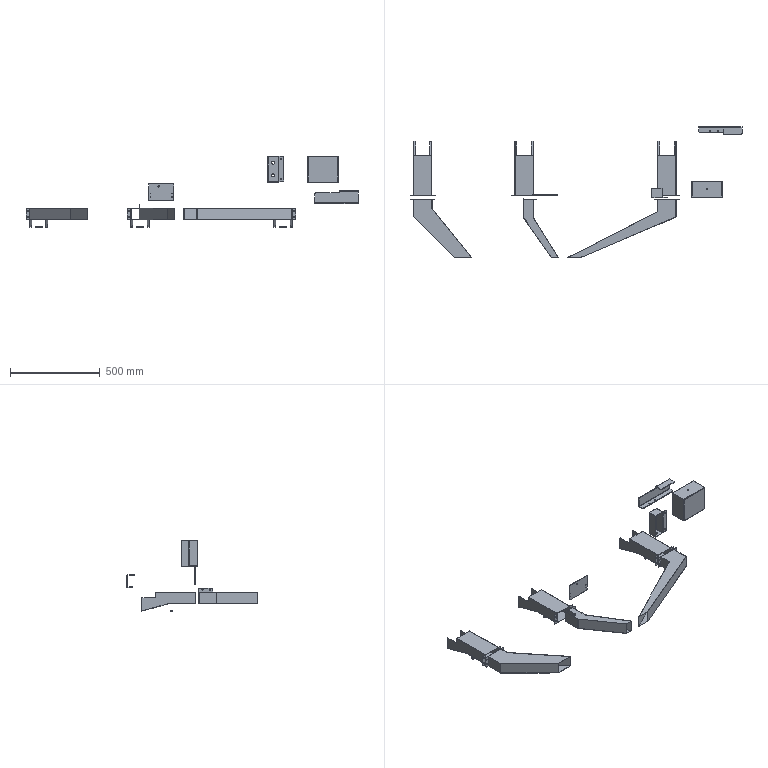Part | NX | 13 solids | 519 faces | box 1848 x 727.9 x 399.48 mm | volume 905518 mm3 | plane 280 | cylinder 167 | cone 72 | commonest cylinder face diameters 6 x78 4.2 x18 6.4 x12 10 x11 3.2 x9 5.2 x9